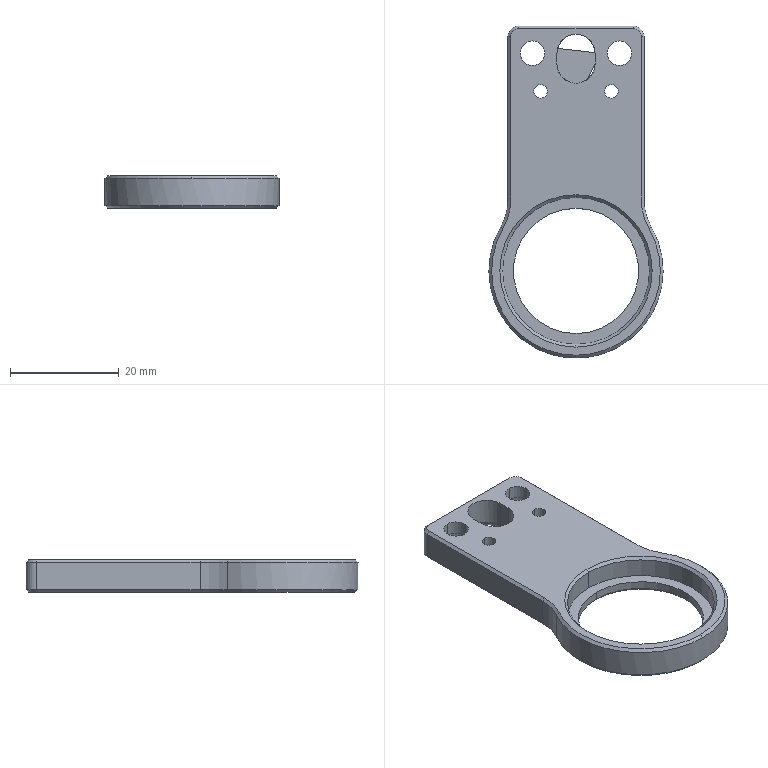NC program | NX | posted with a generic post | part box 32 x 61 x 6 mm
Lines 1 to 1417 of 12533:
N10 G17 G21 G94 G90
(FLOOR_WALL_COPY , TOOL : D80)
N12 T19 M6
N14 G54
N16 G17 G0 G90 X-106. Y0. S5000 M3
N18 G43 Z30. H19
N20 Z7.02
N22 G94 G1 Z4.02 F2000.
N24 X-101.
N26 X40.
N28 X45.
N30 Z7.02
N32 G0 Z30.
N34 X-106.
N36 Z6.04
N38 G1 Z3.04
N40 X-101.
N42 X40.
N44 X45.
N46 Z6.04
N48 G0 Z30.
N50 X-106.
N52 Z5.06
N54 G1 Z2.06
N56 X-101.
N58 X40.
N60 X45.
N62 Z5.06
N64 G0 Z30.
N66 X-106.
N68 Z4.08
N70 G1 Z1.08
N72 X-101.
N74 X40.
N76 X45.
N78 Z4.08
N80 G0 Z30.
N82 X-106.
N84 Z3.1
N86 G1 Z0.1
N88 X-101.
N90 X40.
N92 X45.
N94 Z3.1
N96 G0 Z30.
(FLOOR_WALL_COPY_COPY , TOOL : D80)
N98 X-106.
N100 Z3.
N102 G1 Z0. F1200.
N104 X-101.
N106 X40.
N108 X45.
N110 Z3.
N112 G0 Z30.
N114 M5
(HOLE_MILLING_2 , TOOL : D4)
N116 T11 M6
N118 G54
N120 G17 G0 G90 X-5. Y8. S9500 M3
N122 G43 Z30. H11
N124 Z0.5
N126 G94 G3 X-4.25 Y8.75 R0.75 F1250.
N128 X-5. Y9.5 R0.75
N130 X-5. Y9.5 Z0.1 I0. J-1.5
N132 X-5. Y9.5 Z-0.3 I0. J-1.5
N134 X-5. Y9.5 Z-0.7 I0. J-1.5
N136 X-5. Y9.5 Z-1.1 I0. J-1.5
N138 X-5. Y9.5 Z-1.5 I0. J-1.5
N140 X-5. Y9.5 Z-1.9 I0. J-1.5
N142 X-5. Y9.5 Z-2.3 I0. J-1.5
N144 X-5. Y9.5 Z-2.7 I0. J-1.5
N146 X-5. Y9.5 Z-3.1 I0. J-1.5
N148 X-5. Y9.5 Z-3.5 I0. J-1.5
N150 X-6.5 Y8. R1.5
N152 X-5. Y9.5 R-1.5
N154 X-5.75 Y8.75 R0.75
N156 X-5. Y8. R0.75
N158 G0 Z30.
N160 Y-8.
N162 Z0.5
N164 G3 X-4.25 Y-7.25 R0.75
N166 X-5. Y-6.5 R0.75
N168 X-5. Y-6.5 Z0.1 I0. J-1.5
N170 X-5. Y-6.5 Z-0.3 I0. J-1.5
N172 X-5. Y-6.5 Z-0.7 I0. J-1.5
N174 X-5. Y-6.5 Z-1.1 I0. J-1.5
N176 X-5. Y-6.5 Z-1.5 I0. J-1.5
N178 X-5. Y-6.5 Z-1.9 I0. J-1.5
N180 X-5. Y-6.5 Z-2.3 I0. J-1.5
N182 X-5. Y-6.5 Z-2.7 I0. J-1.5
N184 X-5. Y-6.5 Z-3.1 I0. J-1.5
N186 X-5. Y-6.5 Z-3.5 I0. J-1.5
N188 X-6.5 Y-8. R1.5
N190 X-5. Y-6.5 R-1.5
N192 X-5.75 Y-7.25 R0.75
N194 X-5. Y-8. R0.75
N196 G0 Z30.
(ZLEVEL_PROFILE_COPY_1 , TOOL : D4)
N198 X-20.254 Y1.745
N200 Z1.5
N202 G1 X-23.172 Z1.347 F1000.
N204 X-23.566 Y1.756 Z1.326
N206 X-24.329 Y1.54 Z1.285
N208 X-24.659 Y1.324 Z1.264
N210 Y-1.312 Z1.126
N212 X-24.347 Y-1.531 Z1.106
N214 X-23.552 Y-1.762 Z1.063
N216 X-23.172 Y-1.745 Z1.043
N218 X-4.675 Z0.073
N220 X-4.014 Y-1.476 Z0.036
N222 X-3.512 Y-0.968 Z-0.001
N224 X-3.251 Y-0.304 Z-0.039
N226 X-3.259 Y0.346 Z-0.073
N228 X-3.528 Y0.992 Z-0.11
N230 X-4.026 Y1.484 Z-0.146
N232 X-4.675 Y1.745 Z-0.183
N234 X-5. Z-0.2
N236 X-23.172 F2000.
N238 G3 X-24.659 Y1.324 R2.585
N240 G1 Y-1.312
N242 G3 X-23.172 Y-1.745 R2.404
N244 G1 X-5.
N246 G3 X-3.255 Y0. R1.745
N248 X-5. Y1.745 R1.745
N250 G1 X-6.817 Y1.737 Z-0.208
N252 X-8.634 Y1.729 Z-0.216
N254 X-10.451 Y1.721 Z-0.223
N256 X-12.269 Y1.713 Z-0.231
N258 X-14.086 Y1.706 Z-0.239
N260 X-15.903 Y1.699 Z-0.247
N262 X-17.72 Y1.691 Z-0.254
N264 X-19.537 Y1.684 Z-0.262
N266 X-21.354 Y1.677 Z-0.27
N268 X-23.172 Y1.674 Z-0.278
N270 X-23.696 Y1.617 Z-0.28
N272 X-23.928 Y1.577 Z-0.281
N274 X-24.446 Y1.356 Z-0.283
N276 X-24.575 Y1.296 Z-0.284
N278 X-24.564 Y-1.283 Z-0.295
N280 X-24.164 Y-1.474 Z-0.297
N282 X-23.916 Y-1.557 Z-0.298
N284 X-23.677 Y-1.612 Z-0.299
N286 X-23.172 Y-1.661 Z-0.301
N288 X-21.355 Y-1.644 Z-0.309
N290 X-19.537 Y-1.638 Z-0.317
N292 X-17.72 Y-1.632 Z-0.324
N294 X-15.903 Y-1.626 Z-0.332
N296 X-14.086 Y-1.62 Z-0.34
N298 X-12.269 Y-1.614 Z-0.348
N300 X-10.451 Y-1.609 Z-0.355
N302 X-8.634 Y-1.603 Z-0.363
N304 X-6.817 Y-1.598 Z-0.371
N306 X-5. Y-1.592 Z-0.379
N308 X-4.667 Y-1.556 Z-0.38
N310 X-4.505 Y-1.512 Z-0.381
N312 X-4.229 Y-1.39 Z-0.382
N314 X-4.06 Y-1.281 Z-0.383
N316 X-3.84 Y-1.085 Z-0.384
N318 X-3.709 Y-0.924 Z-0.385
N320 X-3.561 Y-0.67 Z-0.386
N322 X-3.487 Y-0.476 Z-0.387
N324 X-3.426 Y-0.189 Z-0.389
N326 X-3.415 Y0.019 Z-0.39
N328 X-3.446 Y0.306 Z-0.391
N330 X-3.499 Y0.504 Z-0.392
N332 X-3.616 Y0.767 Z-0.393
N334 X-3.727 Y0.939 Z-0.394
N336 X-3.919 Y1.154 Z-0.395
N338 X-4.077 Y1.283 Z-0.396
N340 X-4.325 Y1.429 Z-0.397
N342 X-4.516 Y1.503 Z-0.398
N344 X-4.755 Y1.56 Z-0.399
N346 X-5. Y1.578 Z-0.4
N348 X-6.817 Y1.573 Z-0.408
N350 X-8.634 Y1.568 Z-0.416
N352 X-10.451 Y1.563 Z-0.424
N354 X-12.269 Y1.558 Z-0.432
N356 X-14.086 Y1.553 Z-0.44
N358 X-15.903 Y1.549 Z-0.447
N360 X-17.72 Y1.544 Z-0.455
N362 X-19.537 Y1.54 Z-0.463
N364 X-21.355 Y1.535 Z-0.471
N366 X-23.174 Y1.533 Z-0.479
N368 X-23.59 Y1.504 Z-0.481
N370 X-23.823 Y1.45 Z-0.482
N372 X-24.321 Y1.279 Z-0.484
N374 X-24.374 Y1.251 Z-0.485
N376 X-24.363 Y-1.247 Z-0.495
N378 X-24.28 Y-1.299 Z-0.496
N380 X-23.822 Y-1.44 Z-0.498
N382 X-23.498 Y-1.491 Z-0.499
N384 X-23.172 Y-1.521 Z-0.501
N386 X-21.354 Y-1.516 Z-0.509
N388 X-19.537 Y-1.512 Z-0.517
N390 X-17.72 Y-1.508 Z-0.524
N392 X-15.903 Y-1.504 Z-0.532
N394 X-14.086 Y-1.501 Z-0.54
N396 X-12.269 Y-1.497 Z-0.548
N398 X-10.451 Y-1.494 Z-0.556
N400 X-8.634 Y-1.49 Z-0.564
N402 X-6.817 Y-1.487 Z-0.572
N404 X-5. Y-1.483 Z-0.58
N406 X-4.691 Y-1.45 Z-0.581
N408 X-4.541 Y-1.41 Z-0.582
N410 X-4.285 Y-1.298 Z-0.583
N412 X-4.127 Y-1.197 Z-0.584
N414 X-3.922 Y-1.016 Z-0.585
N416 X-3.8 Y-0.868 Z-0.586
N418 X-3.662 Y-0.633 Z-0.587
N420 X-3.591 Y-0.453 Z-0.588
N422 X-3.532 Y-0.187 Z-0.589
N424 X-3.521 Y0.006 Z-0.59
N426 X-3.547 Y0.275 Z-0.591
N428 X-3.595 Y0.461 Z-0.592
N430 X-3.703 Y0.709 Z-0.593
N432 X-3.807 Y0.871 Z-0.594
N434 X-3.986 Y1.074 Z-0.595
N436 X-4.134 Y1.196 Z-0.596
N438 X-4.367 Y1.334 Z-0.597
N440 X-4.545 Y1.404 Z-0.598
N442 X-4.77 Y1.458 Z-0.599
N444 X-5. Y1.475 Z-0.6
N446 X-6.817 Y1.472 Z-0.608
N448 X-8.634 Y1.469 Z-0.616
N450 X-10.451 Y1.466 Z-0.624
N452 X-12.269 Y1.463 Z-0.632
N454 X-14.086 Y1.461 Z-0.64
N456 X-15.903 Y1.458 Z-0.648
N458 X-17.72 Y1.455 Z-0.656
N460 X-19.537 Y1.453 Z-0.664
N462 X-21.354 Y1.45 Z-0.672
N464 X-23.172 Y1.448 Z-0.68
N466 X-23.219 Y1.454
N468 X-23.496 Y1.433 Z-0.682
N470 X-23.724 Y1.403 Z-0.683
N472 X-23.901 Y1.349
N474 X-24.076 Y1.289 Z-0.684
N476 X-24.174 Y1.243 Z-0.685
N478 X-24.168 Y-0.012 Z-0.69
N480 X-24.162 Y-1.244 Z-0.696
N482 X-24.071 Y-1.281
N484 X-23.898 Y-1.345 Z-0.697
N486 X-23.723 Y-1.398 Z-0.698
N488 X-23.449 Y-1.434 Z-0.699
N490 X-23.173 Y-1.443 Z-0.7
N492 X-21.355 Y-1.439 Z-0.708
N494 X-19.537 Y-1.437 Z-0.716
N496 X-17.72 Y-1.435 Z-0.724
N498 X-15.903 Y-1.433 Z-0.732
N500 X-14.086 Y-1.431 Z-0.74
N502 X-12.269 Y-1.429 Z-0.748
N504 X-10.451 Y-1.427 Z-0.756
N506 X-8.634 Y-1.426 Z-0.764
N508 X-6.817 Y-1.424 Z-0.772
N510 X-5. Y-1.422 Z-0.78
N512 X-4.634 Y-1.374 Z-0.782
N514 X-4.458 Y-1.314 Z-0.783
N516 X-4.168 Y-1.152 Z-0.784
N518 X-3.998 Y-1.008 Z-0.785
N520 X-3.796 Y-0.754 Z-0.787
N522 X-3.69 Y-0.55 Z-0.788
N524 X-3.6 Y-0.238 Z-0.789
N526 X-3.58 Y-0.009 Z-0.79
N528 X-3.616 Y0.316 Z-0.792
N530 X-3.686 Y0.537 Z-0.793
N532 X-3.843 Y0.823 Z-0.794
N534 X-3.993 Y1. Z-0.795
N536 X-4.248 Y1.204 Z-0.797
N538 X-4.455 Y1.31 Z-0.798
N540 X-4.722 Y1.391 Z-0.799
N542 X-5. Y1.418 Z-0.8
N544 X-6.827 Y1.417 Z-0.808
N546 X-8.653 Y1.415 Z-0.816
N548 X-10.48 Y1.414 Z-0.824
N550 X-12.307 Y1.413 Z-0.833
N552 X-14.133 Y1.412 Z-0.841
N554 X-15.96 Y1.41 Z-0.849
N556 X-17.787 Y1.409 Z-0.857
N558 X-19.613 Y1.408 Z-0.865
N560 X-21.356 Y1.407 Z-0.873
N562 X-23.098 Y1.406 Z-0.881
N564 X-23.182 Y1.414
N566 X-23.266 Y1.409
N568 X-23.466 Y1.383 Z-0.882
N570 X-23.665 Y1.35 Z-0.883
N572 X-23.931 Y1.263 Z-0.885
N574 X-23.974 Y1.245
N576 X-23.963 Y-1.245 Z-0.896
N578 X-23.909 Y-1.268
N580 X-23.617 Y-1.355 Z-0.897
N582 X-23.396 Y-1.391 Z-0.898
N584 X-23.064 Y-1.405 Z-0.9
N586 X-21.301 Y-1.404 Z-0.908
N588 X-19.537 Y-1.403 Z-0.916
N590 X-17.72 Z-0.924
N592 X-15.903 Y-1.402 Z-0.932
N594 X-14.086 Z-0.94
N596 X-12.269 Y-1.401 Z-0.948
N598 X-10.451 Z-0.956
N600 X-8.634 Z-0.964
N602 X-6.817 Y-1.4 Z-0.972
N604 X-5. Z-0.98
N606 X-4.638 Y-1.353 Z-0.982
N608 X-4.465 Y-1.294 Z-0.983
N610 X-4.178 Y-1.133 Z-0.984
N612 X-4.011 Y-0.991 Z-0.985
N614 X-3.81 Y-0.738 Z-0.987
N616 X-3.707 Y-0.537 Z-0.988
N618 X-3.619 Y-0.228 Z-0.989
N620 X-3.6 Y-0.002 Z-0.99
N622 X-3.636 Y0.317 Z-0.992
N624 X-3.706 Y0.535 Z-0.993
N626 X-3.862 Y0.815 Z-0.994
N628 X-4.009 Y0.989 Z-0.995
N630 X-4.261 Y1.189 Z-0.997
N632 X-4.464 Y1.293 Z-0.998
N634 X-5. Y1.401 Z-1.
N636 X-6.81 Y1.4 Z-1.008
N638 X-23.098 Z-1.081
N640 X-23.287 Y1.368 Z-1.082
N642 X-23.475 Y1.328 Z-1.083
N644 X-23.774 Y1.242 Z-1.085
N646 X-23.763 Y-1.234 Z-1.096
N648 X-23.732 Y-1.253
N650 X-23.459 Y-1.331 Z-1.097
N652 X-23.262 Y-1.369 Z-1.098
N654 X-23.064 Y-1.4 Z-1.099
N656 X-22.931 Z-1.1
N658 X-5. Z-1.18
N660 X-4.638 Y-1.352 Z-1.182
N662 X-4.464 Y-1.293 Z-1.183
N664 X-4.178 Y-1.133 Z-1.184
N666 X-4.01 Y-0.99 Z-1.185
N668 X-3.81 Y-0.738 Z-1.187
N670 X-3.707 Y-0.536 Z-1.188
N672 X-3.619 Y-0.227 Z-1.189
N674 X-3.6 Y0. Z-1.19
N676 X-3.637 Y0.319 Z-1.192
N678 X-3.707 Y0.536 Z-1.193
N680 X-3.862 Y0.816 Z-1.194
N682 X-4.01 Y0.99 Z-1.195
N684 X-4.261 Y1.189 Z-1.197
N686 X-4.464 Y1.293 Z-1.198
N688 X-4.727 Y1.373 Z-1.199
N690 X-5. Y1.4 Z-1.2
N692 X-19.372 Z-1.265
N694 X-21.168 Z-1.273
N696 X-22.964 Y1.391 Z-1.282
N698 X-23.137 Y1.376
N700 X-23.311 Y1.33 Z-1.283
N702 X-23.574 Y1.238 Z-1.284
N704 X-23.563 Y-1.234 Z-1.296
N706 X-23.469 Y-1.267
N708 X-23.386 Y-1.306 Z-1.297
N710 X-23.297 Y-1.328
N712 X-22.93 Y-1.389 Z-1.299
N714 X-21.138 Y-1.4 Z-1.307
N716 X-19.345 Z-1.315
N718 X-8.586 Z-1.364
N720 X-6.793 Z-1.372
N722 X-5. Z-1.38
N724 X-4.624 Y-1.349 Z-1.382
N726 X-4.444 Y-1.285 Z-1.383
N728 X-4.149 Y-1.112 Z-1.384
N730 X-3.979 Y-0.958 Z-1.385
N732 X-3.783 Y-0.692 Z-1.387
N734 X-3.682 Y-0.473 Z-1.388
N736 X-3.611 Y-0.172 Z-1.389
N738 X-3.601 Y0.053 Z-1.39
N740 X-3.648 Y0.362 Z-1.392
N742 X-3.722 Y0.573 Z-1.393
N744 X-3.882 Y0.842 Z-1.394
N746 X-4.029 Y1.009 Z-1.395
N748 X-4.277 Y1.199 Z-1.397
N750 X-4.477 Y1.298 Z-1.398
N752 X-4.733 Y1.374 Z-1.399
N754 X-5. Y1.4 Z-1.4
N756 X-19.215 Z-1.465
N758 X-20.991 Z-1.473
N760 X-22.766 Y1.382 Z-1.481
N762 X-23.113 Y1.329 Z-1.483
N764 X-23.193 Y1.304
N766 X-23.273 Y1.278 Z-1.484
N768 X-23.374 Y1.237
N770 X-23.363 Y-1.237 Z-1.496
N772 X-23.272 Y-1.277
N774 X-22.827 Y-1.371 Z-1.498
N776 X-21.047 Y-1.4 Z-1.506
N778 X-19.266 Z-1.515
N780 X-8.566 Z-1.564
N782 X-6.783 Z-1.572
N784 X-5. Z-1.58
N786 X-4.624 Y-1.349 Z-1.582
N788 X-4.444 Y-1.285 Z-1.583
N790 X-4.149 Y-1.112 Z-1.584
N792 X-3.979 Y-0.958 Z-1.585
N794 X-3.783 Y-0.692 Z-1.587
N796 X-3.682 Y-0.473 Z-1.588
N798 X-3.611 Y-0.172 Z-1.589
N800 X-3.601 Y0.053 Z-1.59
N802 X-3.648 Y0.362 Z-1.592
N804 X-3.722 Y0.573 Z-1.593
N806 X-3.882 Y0.842 Z-1.594
N808 X-4.029 Y1.009 Z-1.595
N810 X-4.277 Y1.199 Z-1.597
N812 X-4.477 Y1.298 Z-1.598
N814 X-4.733 Y1.374 Z-1.599
N816 X-5. Y1.4 Z-1.6
N818 X-18.938 Z-1.664
N820 X-20.68 Z-1.673
N822 X-22.421 Y1.387 Z-1.681
N824 X-22.842 Y1.339 Z-1.683
N826 X-22.96 Y1.319
N828 X-23.174 Y1.237 Z-1.684
N830 X-23.163 Y-1.236 Z-1.696
N832 X-23.069 Y-1.275
N834 X-22.951 Y-1.318 Z-1.697
N836 X-22.827 Y-1.338
N838 X-22.389 Y-1.39 Z-1.699
N840 X-20.651 Y-1.4 Z-1.707
N842 X-18.912 Z-1.715
N844 X-8.478 Z-1.764
N846 X-6.739 Z-1.772
N848 X-5. Z-1.78
N850 X-4.624 Y-1.349 Z-1.782
N852 X-4.444 Y-1.285
N854 X-4.149 Y-1.112 Z-1.784
N856 X-3.979 Y-0.958 Z-1.785
N858 X-3.783 Y-0.692 Z-1.787
N860 X-3.682 Y-0.473 Z-1.788
N862 X-3.611 Y-0.172 Z-1.789
N864 X-3.601 Y0.053 Z-1.79
N866 X-3.648 Y0.362 Z-1.792
N868 X-3.722 Y0.573 Z-1.793
N870 X-3.882 Y0.842 Z-1.794
N872 X-4.029 Y1.009 Z-1.795
N874 X-4.277 Y1.199 Z-1.797
N876 X-4.477 Y1.298 Z-1.798
N878 X-4.733 Y1.374 Z-1.799
N880 X-5. Y1.4 Z-1.8
N882 X-18.782 Z-1.864
N884 X-20.504 Z-1.872
N886 X-22.224 Y1.375 Z-1.88
N888 X-22.434 Y1.35 Z-1.881
N890 X-22.644 Y1.329 Z-1.882
N892 X-22.931 Y1.257 Z-1.884
N894 X-22.975 Y1.236
N896 X-22.969 Y-0.047 Z-1.89
N898 X-22.961 Y-1.24 Z-1.896
N900 X-22.917 Y-1.257
N902 X-22.53 Y-1.337 Z-1.898
N904 X-22.265 Y-1.367 Z-1.899
N906 X-21.999 Y-1.386 Z-1.9
N908 X-20.3 Y-1.4 Z-1.908
N910 X-18.6 Z-1.916
N912 X-8.4 Z-1.964
N914 X-6.7 Z-1.972
N916 X-5. Z-1.98
N918 X-4.624 Y-1.349 Z-1.981
N920 X-4.444 Y-1.285 Z-1.982
N922 X-4.149 Y-1.112 Z-1.984
N924 X-3.979 Y-0.958 Z-1.985
N926 X-3.783 Y-0.692 Z-1.986
N928 X-3.682 Y-0.473 Z-1.988
N930 X-3.611 Y-0.172 Z-1.989
N932 X-3.601 Y0.053 Z-1.99
N934 X-3.648 Y0.362 Z-1.991
N936 X-3.722 Y0.573 Z-1.993
N938 X-3.882 Y0.842 Z-1.994
N940 X-4.029 Y1.009 Z-1.995
N942 X-4.277 Y1.199 Z-1.996
N944 X-4.477 Y1.298 Z-1.998
N946 X-4.733 Y1.374 Z-1.999
N948 X-5. Y1.4 Z-2.
N950 X-6.288 Z-2.006
N952 X-7.576 Z-2.012
N954 X-7.961 Z-2.014
N956 X-8.346 Z-2.016
N958 X-10.019 Z-2.024
N960 X-11.692 Z-2.032
N962 X-13.365 Z-2.039
N964 X-15.037 Y1.399 Z-2.047
N966 X-16.71 Z-2.055
N968 X-18.383 Z-2.063
N970 X-19.675 Z-2.069
N972 X-20.967 Y1.392 Z-2.075
N974 X-21.347 Y1.384 Z-2.077
N976 X-21.728 Y1.369 Z-2.079
N978 X-22.015 Y1.356 Z-2.08
N980 X-22.297 Y1.338 Z-2.082
N982 X-22.714 Y1.252 Z-2.084
N984 X-22.775 Y1.227
N986 X-22.763 Y-1.225 Z-2.096
N988 X-22.703 Y-1.251
N990 X-22.296 Y-1.336 Z-2.098
N992 X-22.053 Y-1.351 Z-2.099
N994 X-21.727 Y-1.366 Z-2.1
N996 X-21.328 Y-1.381 Z-2.102
N998 X-20.929 Y-1.395 Z-2.104
N1000 X-19.656 Y-1.397 Z-2.11
N1002 X-18.383 Y-1.396 Z-2.116
N1004 X-16.71 Z-2.124
N1006 X-15.037 Y-1.395 Z-2.132
N1008 X-13.365 Z-2.14
N1010 X-11.692 Y-1.394 Z-2.148
N1012 X-10.019 Z-2.156
N1014 X-8.346 Y-1.393 Z-2.164
N1016 X-7.972 Z-2.165
N1018 X-7.598 Z-2.167
N1020 X-6.299 Y-1.4 Z-2.173
N1022 X-5. Z-2.179
N1024 X-4.624 Y-1.349 Z-2.181
N1026 X-4.444 Y-1.285 Z-2.182
N1028 X-4.149 Y-1.112 Z-2.184
N1030 X-3.979 Y-0.958 Z-2.185
N1032 X-3.783 Y-0.692 Z-2.186
N1034 X-3.682 Y-0.473 Z-2.187
N1036 X-3.611 Y-0.172 Z-2.189
N1038 X-3.601 Y0.053 Z-2.19
N1040 X-3.648 Y0.362 Z-2.191
N1042 X-3.722 Y0.573 Z-2.192
N1044 X-3.882 Y0.842 Z-2.194
N1046 X-4.029 Y1.009 Z-2.195
N1048 X-4.277 Y1.199 Z-2.196
N1050 X-4.477 Y1.298 Z-2.197
N1052 X-4.733 Y1.374 Z-2.199
N1054 X-5. Y1.4 Z-2.2
N1056 X-7.135 Z-2.21
N1058 X-7.355 Y1.389 Z-2.211
N1060 X-7.576 Y1.388 Z-2.212
N1062 X-7.761 Z-2.213
N1064 X-7.945 Z-2.214
N1066 X-9.427 Y1.387 Z-2.221
N1068 X-10.908 Y1.386 Z-2.228
N1070 X-12.574 Y1.385 Z-2.236
N1072 X-14.239 Y1.384 Z-2.244
N1074 X-15.905 Y1.383 Z-2.252
N1076 X-17.571 Y1.382 Z-2.26
N1078 X-19.236 Y1.381 Z-2.268
N1080 X-20.902 Y1.371 Z-2.276
N1082 X-21.405 Y1.354 Z-2.278
N1084 X-22.012 Y1.32 Z-2.281
N1086 X-22.505 Y1.231 Z-2.283
N1088 X-22.575 Y1.202 Z-2.284
N1090 X-22.563 Y-1.198 Z-2.295
N1092 X-22.499 Y-1.227 Z-2.296
N1094 X-22.049 Y-1.315 Z-2.298
N1096 X-21.954 Y-1.32
N1098 X-21.441 Y-1.35 Z-2.301
N1100 X-20.929 Y-1.361 Z-2.303
N1102 X-19.263 Y-1.374 Z-2.311
N1104 X-17.596 Y-1.373 Z-2.319
N1106 X-15.93 Y-1.372 Z-2.327
N1108 X-14.263 Y-1.37 Z-2.335
N1110 X-12.597 Y-1.369 Z-2.343
N1112 X-10.93 Y-1.367 Z-2.351
N1114 X-9.264 Y-1.366 Z-2.359
N1116 X-7.598 Y-1.372 Z-2.367
N1118 X-7.47 Y-1.378
N1120 X-7.343 Y-1.383 Z-2.368
N1122 X-7.225 Y-1.386 Z-2.369
N1124 X-7.108 Y-1.395
N1126 X-6.054 Y-1.4 Z-2.374
N1128 X-5. Z-2.379
N1130 X-4.624 Y-1.349 Z-2.381
N1132 X-4.444 Y-1.285 Z-2.382
N1134 X-4.149 Y-1.112 Z-2.383
N1136 X-3.979 Y-0.958 Z-2.385
N1138 X-3.783 Y-0.692 Z-2.386
N1140 X-3.682 Y-0.473 Z-2.387
N1142 X-3.611 Y-0.172 Z-2.389
N1144 X-3.601 Y0.053 Z-2.39
N1146 X-3.648 Y0.362 Z-2.391
N1148 X-3.722 Y0.573 Z-2.392
N1150 X-3.882 Y0.842 Z-2.394
N1152 X-4.029 Y1.009 Z-2.395
N1154 X-4.277 Y1.199 Z-2.396
N1156 X-4.477 Y1.298 Z-2.397
N1158 X-4.733 Y1.374 Z-2.399
N1160 X-5. Y1.4 Z-2.4
N1162 X-6.083 Z-2.405
N1164 X-7.165 Y1.389 Z-2.41
N1166 X-7.277 Y1.38 Z-2.411
N1168 X-7.572 Y1.37 Z-2.412
N1170 X-7.987 Y1.353 Z-2.414
N1172 X-8.236 Y1.354 Z-2.416
N1174 X-8.486 Z-2.417
N1176 X-9.851 Y1.352 Z-2.423
N1178 X-11.215 Y1.351 Z-2.43
N1180 X-12.83 Y1.349 Z-2.438
N1182 X-14.444 Y1.347 Z-2.446
N1184 X-16.058 Y1.345 Z-2.453
N1186 X-17.673 Y1.343 Z-2.461
N1188 X-19.287 Y1.341 Z-2.469
N1190 X-20.901 Y1.336 Z-2.477
N1192 X-21.403 Y1.313 Z-2.479
N1194 X-21.903 Y1.265 Z-2.482
N1196 X-22.335 Y1.184 Z-2.484
N1198 X-22.375 Y1.166
N1200 X-22.369 Y-0.034 Z-2.49
N1202 X-22.363 Y-1.162 Z-2.495
N1204 X-22.319 Y-1.182
N1206 X-21.945 Y-1.254 Z-2.497
N1208 X-21.438 Y-1.305 Z-2.5
N1210 X-20.929 Y-1.328 Z-2.502
N1212 X-19.231 Y-1.33 Z-2.51
N1214 X-17.532 Y-1.328 Z-2.518
N1216 X-15.834 Y-1.326 Z-2.527
N1218 X-14.136 Y-1.323 Z-2.535
N1220 X-12.438 Y-1.321 Z-2.543
N1222 X-10.739 Y-1.318 Z-2.551
N1224 X-9.612 Y-1.317 Z-2.557
N1226 X-8.484 Y-1.313 Z-2.562
N1228 X-7.914 Y-1.328 Z-2.565
N1230 X-7.345 Y-1.374 Z-2.568
N1232 X-7.172 Y-1.387
N1234 X-7. Y-1.4 Z-2.569
N1236 X-5. Z-2.579
N1238 X-4.624 Y-1.349 Z-2.581
N1240 X-4.444 Y-1.285 Z-2.582
N1242 X-4.149 Y-1.112 Z-2.583
N1244 X-3.979 Y-0.958 Z-2.584
N1246 X-3.783 Y-0.692 Z-2.586
N1248 X-3.682 Y-0.473 Z-2.587
N1250 X-3.611 Y-0.172 Z-2.589
N1252 X-3.601 Y0.053 Z-2.59
N1254 X-3.648 Y0.362 Z-2.591
N1256 X-3.722 Y0.573 Z-2.592
N1258 X-3.882 Y0.842 Z-2.594
N1260 X-4.029 Y1.009 Z-2.595
N1262 X-4.277 Y1.199 Z-2.596
N1264 X-4.477 Y1.298 Z-2.597
N1266 X-4.733 Y1.374 Z-2.599
N1268 X-5. Y1.4 Z-2.6
N1270 X-6.109 Z-2.605
N1272 X-7.217 Y1.38 Z-2.611
N1274 X-7.363 Y1.364 Z-2.612
N1276 X-7.613 Y1.334 Z-2.613
N1278 X-7.987 Y1.314 Z-2.615
N1280 X-8.236 Y1.306 Z-2.616
N1282 X-8.486 Y1.298 Z-2.617
N1284 X-8.735 Y1.297 Z-2.618
N1286 X-8.985 Y1.296 Z-2.62
N1288 X-10.291 Y1.294 Z-2.626
N1290 X-11.597 Y1.292 Z-2.632
N1292 X-13.152 Y1.289 Z-2.64
N1294 X-14.707 Y1.286 Z-2.647
N1296 X-16.263 Y1.284 Z-2.655
N1298 X-17.818 Y1.281 Z-2.663
N1300 X-19.373 Y1.278 Z-2.67
N1302 X-20.929 Y1.268 Z-2.678
N1304 X-21.26 Y1.257 Z-2.679
N1306 X-21.589 Y1.221 Z-2.681
N1308 X-22.126 Y1.128 Z-2.684
N1310 X-22.16 Y1.112
N1312 X-22.153 Y-0.042 Z-2.69
N1314 X-22.147 Y-1.109 Z-2.695
N1316 X-22.093 Y-1.13
N1318 X-21.589 Y-1.217 Z-2.698
N1320 X-21.26 Y-1.252 Z-2.699
N1322 X-20.929 Y-1.259 Z-2.701
N1324 X-19.373 Y-1.263 Z-2.708
N1326 X-17.818 Y-1.26 Z-2.716
N1328 X-16.262 Y-1.257 Z-2.724
N1330 X-14.707 Y-1.254 Z-2.731
N1332 X-13.151 Y-1.25 Z-2.739
N1334 X-11.595 Y-1.247 Z-2.746
N1336 X-10.29 Y-1.245 Z-2.753
N1338 X-8.985 Y-1.24 Z-2.759
N1340 X-8.482 Y-1.251 Z-2.762
N1342 X-7.829 Y-1.304 Z-2.765
N1344 X-7.179 Y-1.387 Z-2.768
N1346 X-7.09 Y-1.396
N1348 X-7. Y-1.4 Z-2.769
N1350 X-5. Z-2.779
N1352 X-4.624 Y-1.349 Z-2.78
N1354 X-4.444 Y-1.285 Z-2.781
N1356 X-4.149 Y-1.112 Z-2.783
N1358 X-3.979 Y-0.958 Z-2.784
N1360 X-3.783 Y-0.692 Z-2.786
N1362 X-3.682 Y-0.473 Z-2.787
N1364 X-3.611 Y-0.172 Z-2.788
N1366 X-3.601 Y0.053 Z-2.79
N1368 X-3.648 Y0.362 Z-2.791
N1370 X-3.722 Y0.573 Z-2.792
N1372 X-3.882 Y0.842 Z-2.794
N1374 X-4.029 Y1.009 Z-2.795
N1376 X-4.277 Y1.199 Z-2.796
N1378 X-4.477 Y1.298 Z-2.797
N1380 X-4.733 Y1.374 Z-2.799
N1382 X-5. Y1.4 Z-2.8
N1384 X-6.137 Z-2.806
N1386 X-7.271 Y1.373 Z-2.811
N1388 X-7.362 Y1.358 Z-2.812
N1390 X-7.472 Y1.351
N1392 X-7.654 Y1.307 Z-2.813
N1394 X-7.841 Y1.292 Z-2.814
N1396 X-7.985 Y1.275 Z-2.815
N1398 X-8.485 Y1.241 Z-2.817
N1400 X-8.985 Y1.211 Z-2.82
N1402 X-9.239 Y1.213 Z-2.821
N1404 X-9.493 Z-2.822
N1406 X-11.256 Y1.209 Z-2.831
N1408 X-13.02 Y1.204 Z-2.84
N1410 X-14.997 Y1.199 Z-2.85
N1412 X-16.974 Y1.194 Z-2.859
N1414 X-18.951 Y1.189 Z-2.869
N1416 X-20.928 Y1.171 Z-2.879
N1418 X-21.828 Y1.074 Z-2.883
N1420 X-21.916 Y1.045 Z-2.884
N1422 X-21.909 Y-0.01 Z-2.889
N1424 X-21.903 Y-1.041 Z-2.894
N1426 X-21.899 Y-1.05
N1428 X-21.719 Y-1.082 Z-2.895
N1430 X-21.472 Y-1.12 Z-2.897
N1432 X-21.201 Y-1.147 Z-2.898
N1434 X-20.929 Y-1.16 Z-2.899
N1436 X-18.938 Y-1.168 Z-2.909
N1438 X-16.948 Y-1.163 Z-2.919
N1440 X-14.957 Y-1.157 Z-2.929
N1442 X-12.966 Y-1.152 Z-2.939
N1444 X-11.23 Y-1.147 Z-2.947
N1446 X-9.494 Y-1.142 Z-2.956
N1448 X-8.981 Y-1.146 Z-2.958
N1450 X-8.543 Y-1.189 Z-2.961
N1452 X-8.105 Y-1.233 Z-2.963
N1454 X-7.769 Y-1.282 Z-2.965
N1456 X-7.434 Y-1.341 Z-2.966
N1458 X-7.337 Y-1.358 Z-2.967
N1460 X-7.241 Y-1.378
N1462 X-6.077 Y-1.4 Z-2.973
N1464 X-5. Z-2.978
N1466 X-4.624 Y-1.349 Z-2.98
N1468 X-4.444 Y-1.285 Z-2.981
N1470 X-4.149 Y-1.112 Z-2.983
N1472 X-3.979 Y-0.958 Z-2.984
N1474 X-3.783 Y-0.692 Z-2.986
N1476 X-3.682 Y-0.473 Z-2.987
N1478 X-3.611 Y-0.172 Z-2.988
N1480 X-3.601 Y0.053 Z-2.989
N1482 X-3.648 Y0.362 Z-2.991
N1484 X-3.722 Y0.573 Z-2.992
N1486 X-3.882 Y0.842 Z-2.994
N1488 X-4.029 Y1.009 Z-2.995
N1490 X-4.277 Y1.199 Z-2.996
N1492 X-4.477 Y1.298 Z-2.997
N1494 X-4.733 Y1.374 Z-2.999
N1496 X-5. Y1.4 Z-3.
N1498 X-6.175 Z-3.006
N1500 X-7.339 Y1.356 Z-3.012
N1502 X-7.474 Y1.34 Z-3.013
N1504 X-7.563 Y1.311
N1506 X-7.654 Y1.29 Z-3.014
N1508 X-8.064 Y1.228 Z-3.016
N1510 X-8.475 Y1.17 Z-3.018
N1512 X-8.983 Y1.126 Z-3.02
N1514 X-9.492 Y1.1 Z-3.023
N1516 X-9.752 Z-3.024
N1518 X-10.011 Z-3.025
N1520 X-11.658 Y1.094 Z-3.034
N1522 X-13.305 Y1.089 Z-3.042
N1524 X-15.211 Y1.082 Z-3.052
N1526 X-17.117 Y1.076 Z-3.061
N1528 X-19.023 Y1.069 Z-3.071
N1530 X-20.929 Y1.057 Z-3.081
N1532 X-21.568 Y0.984 Z-3.084
N1534 X-21.636 Y0.968
N1536 X-21.629 Y-0.005 Z-3.089
N1538 X-21.622 Y-0.963 Z-3.094
N1540 X-21.415 Y-0.99 Z-3.095
N1542 X-20.929 Y-1.046 Z-3.097
N1544 X-19.023 Y-1.044 Z-3.107
N1546 X-17.117 Y-1.037 Z-3.117
N1548 X-15.211 Y-1.03 Z-3.126
N1550 X-13.306 Y-1.023 Z-3.136
N1552 X-11.675 Y-1.017 Z-3.144
N1554 X-10.045 Y-1.011 Z-3.152
N1556 X-9.488 Y-1.015 Z-3.155
N1558 X-8.968 Y-1.064 Z-3.158
N1560 X-8.451 Y-1.128 Z-3.16
N1562 X-7.938 Y-1.216 Z-3.163
N1564 X-7.434 Y-1.34 Z-3.166
N1566 X-7.381 Y-1.345
N1568 X-7.332 Y-1.357
N1570 X-6.2 Y-1.4 Z-3.172
N1572 X-5. Z-3.178
N1574 X-4.624 Y-1.349 Z-3.18
N1576 X-4.444 Y-1.285 Z-3.181
N1578 X-4.149 Y-1.112 Z-3.183
N1580 X-3.979 Y-0.958 Z-3.184
N1582 X-3.783 Y-0.692 Z-3.185
N1584 X-3.682 Y-0.473 Z-3.187
N1586 X-3.611 Y-0.172 Z-3.188
N1588 X-3.601 Y0.053 Z-3.189
N1590 X-3.648 Y0.362 Z-3.191
N1592 X-3.722 Y0.573 Z-3.192
N1594 X-3.882 Y0.842 Z-3.193
N1596 X-4.029 Y1.009 Z-3.195
N1598 X-4.277 Y1.199 Z-3.196
N1600 X-4.477 Y1.298 Z-3.197
N1602 X-4.733 Y1.374 Z-3.199
N1604 X-5. Y1.4 Z-3.2
N1606 X-6.176 Z-3.206
N1608 X-7.345 Y1.355 Z-3.212
N1610 X-7.696 Y1.262 Z-3.214
N1612 X-8.271 Y1.155 Z-3.217
N1614 X-8.846 Y1.05 Z-3.22
N1616 X-9.561 Y0.957 Z-3.224
N1618 X-10.01 Y0.948 Z-3.226
N1620 X-10.266 Y0.95 Z-3.227
N1622 X-10.521 Y0.949 Z-3.229
N1624 X-12.086 Y0.942 Z-3.237
N1626 X-13.651 Y0.935 Z-3.245
N1628 X-15.47 Y0.927 Z-3.254
N1630 X-17.29 Y0.919 Z-3.264
N1632 X-19.109 Y0.91 Z-3.273
N1634 X-20.929 Y0.872 Z-3.282
N1636 X-21.307 Y0.864 Z-3.284
N1638 X-21.299 Y0.001 Z-3.289
N1640 X-21.289 Y-0.857 Z-3.293
N1642 X-20.929 Y-0.86 Z-3.295
N1644 X-19.115 Y-0.882 Z-3.304
N1646 X-17.301 Y-0.873 Z-3.314
N1648 X-15.487 Y-0.864 Z-3.323
N1650 X-13.673 Y-0.854 Z-3.332
N1652 X-12.099 Y-0.846 Z-3.341
N1654 X-10.525 Y-0.838 Z-3.349
N1656 X-10.036 Y-0.833 Z-3.351
N1658 X-9.37 Y-0.906 Z-3.355
N1660 X-8.71 Y-1.025 Z-3.358
N1662 X-8.155 Y-1.144 Z-3.361
N1664 X-7.603 Y-1.276 Z-3.364
N1666 X-7.474 Y-1.315 Z-3.365
N1668 X-7.345 Y-1.353
N1670 X-6.279 Y-1.4 Z-3.371
N1672 X-5. Z-3.377
N1674 X-4.624 Y-1.349 Z-3.379
N1676 X-4.444 Y-1.285 Z-3.38
N1678 X-4.149 Y-1.112 Z-3.382
N1680 X-3.979 Y-0.958 Z-3.383
N1682 X-3.783 Y-0.692 Z-3.385
N1684 X-3.682 Y-0.473 Z-3.386
N1686 X-3.611 Y-0.172 Z-3.388
N1688 X-3.601 Y0.053 Z-3.389
N1690 X-3.648 Y0.362 Z-3.391
N1692 X-3.722 Y0.573 Z-3.392
N1694 X-3.882 Y0.842 Z-3.393
N1696 X-4.029 Y1.009 Z-3.395
N1698 X-4.277 Y1.199 Z-3.396
N1700 X-4.477 Y1.298 Z-3.397
N1702 X-4.733 Y1.374 Z-3.399
N1704 X-5. Y1.4 Z-3.4
N1706 X-6.11 Z-3.406
N1708 X-7.219 Y1.38 Z-3.412
N1710 X-7.318 Y1.36
N1712 X-7.541 Y1.29 Z-3.414
N1714 X-8.006 Y1.159 Z-3.416
N1716 X-8.478 Y1.051 Z-3.419
N1718 X-9.552 Y0.825 Z-3.425
N1720 X-10.034 Y0.783 Z-3.427
N1722 X-10.516 Y0.745 Z-3.43
N1724 X-10.81 Y0.75 Z-3.431
N1726 X-11.104 Y0.748 Z-3.433
N1728 X-12.547 Y0.739 Z-3.441
N1730 X-13.99 Y0.73 Z-3.448
N1732 X-15.725 Y0.719 Z-3.457
N1734 X-17.46 Y0.708 Z-3.467
N1736 X-19.132 Y0.697 Z-3.475
N1738 X-20.805 Y0.686 Z-3.484
N1740 X-20.891 Y0.674 Z-3.485
N1742 X-20.903 Y0.665
N1744 X-20.894 Y-0.057 Z-3.489
N1746 X-20.887 Y-0.657 Z-3.492
N1748 X-20.876 Y-0.666
N1750 X-20.793 Y-0.676
N1752 X-19.127 Y-0.665 Z-3.501
N1754 X-17.461 Y-0.653 Z-3.51
N1756 X-15.727 Y-0.641 Z-3.519
N1758 X-13.993 Y-0.629 Z-3.528
N1760 X-12.549 Y-0.618 Z-3.536
N1762 X-11.106 Y-0.608 Z-3.544
N1764 X-10.506 Y-0.602 Z-3.547
N1766 X-9.784 Y-0.703 Z-3.551
N1768 X-9.071 Y-0.852 Z-3.555
N1770 X-8.405 Y-1.028 Z-3.558
N1772 X-7.742 Y-1.215 Z-3.562
N1774 X-7.67 Y-1.238
N1776 X-7.599 Y-1.264 Z-3.563
N1778 X-7.508 Y-1.3
N1780 X-7.417 Y-1.335 Z-3.564
N1782 X-7.243 Y-1.376 Z-3.565
N1784 X-7. Y-1.4 Z-3.566
N1786 X-5. Z-3.577
N1788 X-4.624 Y-1.349 Z-3.579
N1790 X-4.444 Y-1.285 Z-3.58
N1792 X-4.149 Y-1.112 Z-3.582
N1794 X-3.979 Y-0.958 Z-3.583
N1796 X-3.783 Y-0.692 Z-3.585
N1798 X-3.682 Y-0.473 Z-3.586
N1800 X-3.611 Y-0.172 Z-3.587
N1802 X-3.601 Y0.053 Z-3.589
N1804 X-3.648 Y0.362 Z-3.59
N1806 X-3.722 Y0.573 Z-3.592
N1808 X-3.882 Y0.842 Z-3.593
N1810 X-4.029 Y1.009 Z-3.594
N1812 X-4.277 Y1.199 Z-3.596
N1814 X-4.477 Y1.298 Z-3.597
N1816 X-4.733 Y1.374 Z-3.599
N1818 X-5. Y1.4 Z-3.6
N1820 X-6.11 Z-3.606
N1822 X-7.219 Y1.38 Z-3.612
N1824 X-7.351 Y1.353 Z-3.613
N1826 X-7.478 Y1.308 Z-3.614
N1828 X-8.085 Y1.102 Z-3.617
N1830 X-8.705 Y0.926 Z-3.621
N1832 X-9.289 Y0.762 Z-3.624
N1834 X-9.881 Y0.621 Z-3.628
N1836 X-10.331 Y0.533 Z-3.63
N1838 X-10.789 Y0.486 Z-3.633
N1840 X-11.093 Y0.463 Z-3.635
N1842 X-11.408 Y0.466 Z-3.636
N1844 X-11.724 Y0.463 Z-3.638
N1846 X-12.999 Y0.45 Z-3.645
N1848 X-14.275 Y0.438 Z-3.652
N1850 X-15.86 Y0.422 Z-3.661
N1852 X-17.446 Y0.406 Z-3.67
N1854 X-18.905 Y0.391 Z-3.678
N1856 X-20.362 Y0.373 Z-3.686
N1858 X-20.349 Y-0.366 Z-3.69
N1860 X-18.899 Y-0.353 Z-3.698
N1862 X-17.447 Y-0.337 Z-3.706
N1864 X-15.861 Y-0.319 Z-3.714
N1866 X-14.276 Y-0.3 Z-3.723
N1868 X-13.009 Y-0.285 Z-3.73
N1870 X-11.743 Y-0.269 Z-3.737
N1872 X-11.063 Y-0.286 Z-3.741
N1874 X-10.49 Y-0.369 Z-3.744
N1876 X-9.928 Y-0.502 Z-3.747
N1878 X-9.372 Y-0.655 Z-3.751
N1880 X-8.821 Y-0.821 Z-3.754
N1882 X-8.246 Y-1.028 Z-3.757
N1884 X-7.671 Y-1.235 Z-3.761
N1886 X-7.577 Y-1.273
N1888 X-7.482 Y-1.311 Z-3.762
N1890 X-7.254 Y-1.375 Z-3.763
N1892 X-7. Y-1.4 Z-3.765
N1894 X-5. Z-3.776
N1896 X-4.624 Y-1.349 Z-3.778
N1898 X-4.444 Y-1.285 Z-3.779
N1900 X-4.149 Y-1.112 Z-3.781
N1902 X-3.979 Y-0.958 Z-3.782
N1904 X-3.783 Y-0.692 Z-3.784
N1906 X-3.682 Y-0.473 Z-3.785
N1908 X-3.611 Y-0.172 Z-3.787
N1910 X-3.601 Y0.053 Z-3.788
N1912 X-3.648 Y0.362 Z-3.79
N1914 X-3.722 Y0.573 Z-3.791
N1916 X-3.882 Y0.842 Z-3.793
N1918 X-4.029 Y1.009 Z-3.794
N1920 X-4.277 Y1.199 Z-3.796
N1922 X-4.477 Y1.298 Z-3.797
N1924 X-4.733 Y1.374 Z-3.799
N1926 X-5. Y1.4 Z-3.8
N1928 X-6.11 Z-3.809
N1930 X-7.219 Y1.38 Z-3.818
N1932 X-7.285 Y1.368 Z-3.819
N1934 X-7.539 Y1.284 Z-3.821
N1936 X-8.33 Y0.976 Z-3.828
N1938 X-9.13 Y0.689 Z-3.835
N1940 X-9.505 Y0.554 Z-3.839
N1942 X-9.883 Y0.425 Z-3.842
N1944 X-10.546 Y0.214 Z-3.848
N1946 X-11.15 Y0.095 Z-3.855
N1948 X-10.941 Y0.042 Z-3.882
N1950 X-10.962 Y0.005 Z-3.889
N1952 X-10.834 Y-0.041 Z-3.892
N1954 X-10.347 Y-0.049 Z-3.906
N1956 X-10.241 Y-0.074 Z-3.916
N1958 X-10.021 Y-0.321 Z-3.921
N1960 X-9.445 Y-0.521 Z-3.925
N1962 X-8.888 Y-0.737 Z-3.93
N1964 X-8.21 Y-1.007 Z-3.936
N1966 X-7.537 Y-1.289 Z-3.942
N1968 X-7.268 Y-1.372 Z-3.945
N1970 X-7. Y-1.4 Z-3.947
N1972 X-5. Z-3.964
N1974 X-4.624 Y-1.349 Z-3.967
N1976 X-4.444 Y-1.285 Z-3.968
N1978 X-4.149 Y-1.112 Z-3.971
N1980 X-3.979 Y-0.958 Z-3.973
N1982 X-3.783 Y-0.692 Z-3.976
N1984 X-3.682 Y-0.473 Z-3.978
N1986 X-3.611 Y-0.172 Z-3.98
N1988 X-3.601 Y0.053 Z-3.982
N1990 X-3.648 Y0.362 Z-3.985
N1992 X-3.722 Y0.573 Z-3.987
N1994 X-3.882 Y0.842 Z-3.989
N1996 X-4.029 Y1.009 Z-3.991
N1998 X-4.277 Y1.199 Z-3.994
N2000 X-4.477 Y1.298 Z-3.996
N2002 X-4.733 Y1.374 Z-3.998
N2004 X-5. Y1.4 Z-4.
N2006 X-6.11 Z-4.015
N2008 X-7.219 Y1.38 Z-4.03
N2010 X-7.359 Y1.351 Z-4.032
N2012 X-7.601 Y1.26 Z-4.036
N2014 X-7.773 Y1.172 Z-4.038
N2016 X-7.947 Y1.088 Z-4.041
N2018 X-9.438 Y0.411 Z-4.063
N2020 X-9.657 Y0.303 Z-4.066
N2022 X-9.666 Y0.275 Z-4.067
N2024 X-9.67 Y0.196 Z-4.068
N2026 X-9.671 Y-0.011 Z-4.071
N2028 X-9.648 Y-0.272 Z-4.074
N2030 X-9.638 Y-0.303 Z-4.075
N2032 X-9.42 Y-0.408 Z-4.078
N2034 X-9.09 Y-0.557 Z-4.083
N2036 X-8.344 Y-0.907 Z-4.094
N2038 X-7.6 Y-1.263 Z-4.105
N2040 X-7.412 Y-1.338 Z-4.108
N2042 X-7.306 Y-1.364 Z-4.11
N2044 X-7.154 Y-1.39 Z-4.112
N2046 X-7. Y-1.4 Z-4.114
N2048 X-5. Z-4.141
N2050 X-4.624 Y-1.349 Z-4.146
N2052 X-4.444 Y-1.285 Z-4.149
N2054 X-4.149 Y-1.112 Z-4.153
N2056 X-3.979 Y-0.958 Z-4.156
N2058 X-3.783 Y-0.692 Z-4.161
N2060 X-3.682 Y-0.473 Z-4.164
N2062 X-3.611 Y-0.172 Z-4.168
N2064 X-3.601 Y0.053 Z-4.171
N2066 X-3.648 Y0.362 Z-4.175
N2068 X-3.722 Y0.573 Z-4.178
N2070 X-3.882 Y0.842 Z-4.183
N2072 X-4.029 Y1.009 Z-4.186
N2074 X-4.277 Y1.199 Z-4.19
N2076 X-4.477 Y1.298 Z-4.193
N2078 X-4.733 Y1.374 Z-4.196
N2080 X-5. Y1.4 Z-4.2
N2082 X-6.11 Z-4.216
N2084 X-7.219 Y1.38 Z-4.231
N2086 X-7.392 Y1.339 Z-4.234
N2088 X-7.665 Y1.23 Z-4.238
N2090 X-7.805 Y1.15 Z-4.24
N2092 X-7.869 Y1.132 Z-4.241
N2094 X-9.149 Y0.409 Z-4.262
N2096 X-9.295 Y0.325 Z-4.265
N2098 X-9.309 Y0.151 Z-4.267
N2100 X-9.311 Y0. Z-4.269
N2102 X-9.281 Y-0.323 Z-4.274
N2104 X-9.213 Y-0.364 Z-4.275
N2106 X-9.044 Y-0.469 Z-4.278
N2108 X-7.668 Y-1.229 Z-4.3
N2110 X-7.462 Y-1.318 Z-4.303
N2112 X-7.343 Y-1.355 Z-4.305
N2114 X-7.172 Y-1.386 Z-4.307
N2116 X-7. Y-1.4 Z-4.31
N2118 X-5. Z-4.338
N2120 X-4.624 Y-1.349 Z-4.343
N2122 X-4.444 Y-1.285 Z-4.346
N2124 X-4.149 Y-1.112 Z-4.351
N2126 X-3.979 Y-0.958 Z-4.354
N2128 X-3.783 Y-0.692 Z-4.359
N2130 X-3.682 Y-0.473 Z-4.362
N2132 X-3.611 Y-0.172 Z-4.367
N2134 X-3.601 Y0.053 Z-4.37
N2136 X-3.648 Y0.362 Z-4.374
N2138 X-3.722 Y0.573 Z-4.377
N2140 X-3.882 Y0.842 Z-4.382
N2142 X-4.029 Y1.009 Z-4.385
N2144 X-4.277 Y1.199 Z-4.389
N2146 X-4.477 Y1.298 Z-4.392
N2148 X-4.733 Y1.374 Z-4.396
N2150 X-5. Y1.4 Z-4.4
N2152 X-6.11 Z-4.416
N2154 X-7.219 Y1.38 Z-4.432
N2156 X-7.359 Y1.351 Z-4.435
N2158 X-7.748 Y1.181 Z-4.441
N2160 X-7.804 Y1.148 Z-4.442
N2162 X-7.864 Y1.121 Z-4.443
N2164 X-8.138 Y0.943 Z-4.447
N2166 X-8.415 Y0.77 Z-4.452
N2168 X-8.685 Y0.591 Z-4.457
N2170 X-8.951 Y0.405 Z-4.462
N2172 X-9.04 Y0.342 Z-4.463
N2174 X-9.059 Y0.165 Z-4.466
N2176 X-9.063 Y0. Z-4.468
N2178 X-9.04 Y-0.278 Z-4.472
N2180 X-9.032 Y-0.328 Z-4.473
N2182 X-9.021 Y-0.354
N2184 X-8.949 Y-0.409 Z-4.475
N2186 X-8.833 Y-0.485 Z-4.477
N2188 X-8.382 Y-0.776 Z-4.485
N2190 X-7.931 Y-1.066 Z-4.492
N2192 X-7.871 Y-1.104 Z-4.493
N2194 X-7.729 Y-1.193 Z-4.496
N2196 X-7.512 Y-1.299 Z-4.499
N2198 X-7.377 Y-1.346 Z-4.502
N2200 X-7.216 Y-1.381 Z-4.504
N2202 X-7. Y-1.4 Z-4.507
N2204 X-5. Z-4.536
N2206 X-4.624 Y-1.349 Z-4.542
N2208 X-4.444 Y-1.285 Z-4.545
N2210 X-4.149 Y-1.112 Z-4.549
N2212 X-3.979 Y-0.958 Z-4.553
N2214 X-3.783 Y-0.692 Z-4.558
N2216 X-3.682 Y-0.473 Z-4.561
N2218 X-3.611 Y-0.172 Z-4.566
N2220 X-3.601 Y0.053 Z-4.569
N2222 X-3.648 Y0.362 Z-4.573
N2224 X-3.722 Y0.573 Z-4.577
N2226 X-3.882 Y0.842 Z-4.581
N2228 X-4.029 Y1.009 Z-4.584
N2230 X-4.277 Y1.199 Z-4.589
N2232 X-4.477 Y1.298 Z-4.592
N2234 X-4.733 Y1.374 Z-4.596
N2236 X-5. Y1.4 Z-4.6
N2238 X-6.11 Z-4.617
N2240 X-7.219 Y1.38 Z-4.633
N2242 X-7.352 Y1.352 Z-4.635
N2244 X-7.525 Y1.29 Z-4.638
N2246 X-7.673 Y1.225 Z-4.64
N2248 X-7.811 Y1.141 Z-4.643
N2250 X-7.9 Y1.08 Z-4.644
N2252 X-7.988 Y1.018 Z-4.646
N2254 X-8.365 Y0.749 Z-4.653
N2256 X-8.578 Y0.597 Z-4.657
N2258 X-8.771 Y0.424 Z-4.661
N2260 X-8.848 Y0.352 Z-4.662
N2262 X-8.872 Y0.156 Z-4.665
N2264 X-8.877 Y-0.013 Z-4.668
N2266 X-8.851 Y-0.286 Z-4.672
N2268 X-8.84 Y-0.348 Z-4.673
N2270 X-8.825 Y-0.37
N2272 X-8.775 Y-0.421 Z-4.674
N2274 X-8.395 Y-0.721 Z-4.681
N2276 X-8. Y-1.007 Z-4.689
N2278 X-7.97 Y-1.043
N2280 X-7.927 Y-1.06 Z-4.69
N2282 X-7.868 Y-1.098 Z-4.691
N2284 X-7.812 Y-1.139 Z-4.692
N2286 X-7.567 Y-1.278 Z-4.696
N2288 X-7.424 Y-1.332 Z-4.699
N2290 X-7.238 Y-1.377 Z-4.701
N2292 X-7. Y-1.4 Z-4.705
N2294 X-5. Z-4.735
N2296 X-4.624 Y-1.349 Z-4.74
N2298 X-4.444 Y-1.285 Z-4.743
N2300 X-4.149 Y-1.112 Z-4.748
N2302 X-3.979 Y-0.958 Z-4.752
N2304 X-3.783 Y-0.692 Z-4.757
N2306 X-3.682 Y-0.473 Z-4.76
N2308 X-3.611 Y-0.172 Z-4.765
N2310 X-3.601 Y0.053 Z-4.768
N2312 X-3.648 Y0.362 Z-4.773
N2314 X-3.722 Y0.573 Z-4.776
N2316 X-3.882 Y0.842 Z-4.781
N2318 X-4.029 Y1.009 Z-4.784
N2320 X-4.277 Y1.199 Z-4.789
N2322 X-4.477 Y1.298 Z-4.792
N2324 X-4.733 Y1.374 Z-4.796
N2326 X-5. Y1.4 Z-4.8
N2328 X-6.11 Z-4.817
N2330 X-7.219 Y1.38 Z-4.834
N2332 X-7.369 Y1.347 Z-4.836
N2334 X-7.55 Y1.28 Z-4.839
N2336 X-7.709 Y1.206 Z-4.842
N2338 X-7.855 Y1.109 Z-4.844
N2340 X-7.918 Y1.059 Z-4.846
N2342 X-7.983 Y1.01 Z-4.847
N2344 X-8.629 Y0.455 Z-4.86
N2346 X-8.695 Y0.373 Z-4.861
N2348 X-8.714 Y0.266 Z-4.863
N2350 X-8.732 Y0. Z-4.867
N2352 X-8.702 Y-0.306 Z-4.872
N2354 X-8.679 Y-0.394 Z-4.873
N2356 X-8.619 Y-0.456 Z-4.874
N2358 X-7.994 Y-0.999 Z-4.887
N2360 X-7.925 Y-1.053 Z-4.888
N2362 X-7.857 Y-1.107 Z-4.89
N2364 X-7.609 Y-1.261 Z-4.894
N2366 X-7.451 Y-1.323 Z-4.897
N2368 X-7.249 Y-1.375 Z-4.9
N2370 X-7. Y-1.4 Z-4.903
N2372 X-5. Z-4.934
N2374 X-4.624 Y-1.349 Z-4.939
N2376 X-4.444 Y-1.285 Z-4.942
N2378 X-4.149 Y-1.112 Z-4.948
N2380 X-3.979 Y-0.958 Z-4.951
N2382 X-3.783 Y-0.692 Z-4.956
N2384 X-3.682 Y-0.473 Z-4.96
N2386 X-3.611 Y-0.172 Z-4.964
N2388 X-3.601 Y0.053 Z-4.968
N2390 X-3.648 Y0.362 Z-4.972
N2392 X-3.722 Y0.573 Z-4.976
N2394 X-3.882 Y0.842 Z-4.98
N2396 X-4.029 Y1.009 Z-4.984
N2398 X-4.277 Y1.199 Z-4.989
N2400 X-4.477 Y1.298 Z-4.992
N2402 X-4.733 Y1.374 Z-4.996
N2404 X-5. Y1.4 Z-5.
N2406 X-6.11 Z-5.017
N2408 X-7.219 Y1.379 Z-5.034
N2410 X-7.401 Y1.336 Z-5.037
N2412 X-7.589 Y1.264 Z-5.04
N2414 X-7.754 Y1.177 Z-5.043
N2416 X-7.921 Y1.054 Z-5.046
N2418 X-7.988 Y0.992 Z-5.048
N2420 X-8.146 Y0.868 Z-5.051
N2422 X-8.283 Y0.72 Z-5.054
N2424 X-8.435 Y0.559 Z-5.057
N2426 X-8.574 Y0.39 Z-5.061
N2428 X-8.598 Y0.274 Z-5.062
N2430 X-8.619 Y0. Z-5.067
N2432 X-8.591 Y-0.289 Z-5.071
N2434 X-8.57 Y-0.383 Z-5.073
N2436 X-8.446 Y-0.551 Z-5.076
N2438 X-8.377 Y-0.63 Z-5.077
N2440 X-8.232 Y-0.775 Z-5.081
N2442 X-7.923 Y-1.053 Z-5.087
N2444 X-7.661 Y-1.23 Z-5.092
N2446 X-7.49 Y-1.306 Z-5.095
N2448 X-7.275 Y-1.37 Z-5.098
N2450 X-7. Y-1.4 Z-5.102
N2452 X-5. Z-5.133
N2454 X-4.624 Y-1.349 Z-5.139
N2456 X-4.444 Y-1.285 Z-5.142
N2458 X-4.149 Y-1.112 Z-5.147
N2460 X-3.979 Y-0.958 Z-5.15
N2462 X-3.783 Y-0.692 Z-5.155
N2464 X-3.682 Y-0.473 Z-5.159
N2466 X-3.611 Y-0.172 Z-5.164
N2468 X-3.601 Y0.053 Z-5.167
N2470 X-3.648 Y0.362 Z-5.172
N2472 X-3.722 Y0.573 Z-5.175
N2474 X-3.882 Y0.842 Z-5.18
N2476 X-4.029 Y1.009 Z-5.184
N2478 X-4.277 Y1.199 Z-5.188
N2480 X-4.477 Y1.298 Z-5.192
N2482 X-4.733 Y1.374 Z-5.196
N2484 X-5. Y1.4 Z-5.2
N2486 X-6.11 Z-5.217
N2488 X-7.219 Y1.379 Z-5.234
N2490 X-7.434 Y1.323 Z-5.238
N2492 X-7.631 Y1.247 Z-5.241
N2494 X-7.782 Y1.159 Z-5.244
N2496 X-7.987 Y0.992 Z-5.248
N2498 X-8.059 Y0.92 Z-5.25
N2500 X-8.163 Y0.812 Z-5.252
N2502 X-8.268 Y0.705 Z-5.254
N2504 X-8.427 Y0.499 Z-5.258
N2506 X-8.468 Y0.429 Z-5.26
N2508 X-8.514 Y0.245 Z-5.262
N2510 X-8.532 Y-0.005 Z-5.266
N2512 X-8.504 Y-0.284 Z-5.271
N2514 X-8.473 Y-0.418 Z-5.273
N2516 X-8.287 Y-0.695 Z-5.278
N2518 X-8.169 Y-0.804 Z-5.28
N2520 X-7.99 Y-0.99 Z-5.284
N2522 X-7.714 Y-1.2 Z-5.29
N2524 X-7.533 Y-1.291 Z-5.293
N2526 X-7.306 Y-1.363 Z-5.297
N2528 X-7. Y-1.4 Z-5.301
N2530 X-5. Z-5.332
N2532 X-4.624 Y-1.349 Z-5.338
N2534 X-4.444 Y-1.285 Z-5.341
N2536 X-4.149 Y-1.112 Z-5.346
N2538 X-3.979 Y-0.958 Z-5.35
N2540 X-3.783 Y-0.692 Z-5.355
N2542 X-3.682 Y-0.473 Z-5.359
N2544 X-3.611 Y-0.172 Z-5.363
N2546 X-3.601 Y0.053 Z-5.367
N2548 X-3.648 Y0.362 Z-5.372
N2550 X-3.722 Y0.573 Z-5.375
N2552 X-3.882 Y0.842 Z-5.38
N2554 X-4.029 Y1.009 Z-5.383
N2556 X-4.277 Y1.199 Z-5.388
N2558 X-4.477 Y1.298 Z-5.392
N2560 X-4.733 Y1.374 Z-5.396
N2562 X-5. Y1.4 Z-5.4
N2564 X-6.11 Z-5.417
N2566 X-7.219 Y1.379 Z-5.435
N2568 X-7.464 Y1.312 Z-5.439
N2570 X-7.676 Y1.223 Z-5.442
N2572 X-7.843 Y1.117 Z-5.445
N2574 X-8.057 Y0.918 Z-5.45
N2576 X-8.134 Y0.828 Z-5.452
N2578 X-8.2 Y0.753 Z-5.453
N2580 X-8.263 Y0.676 Z-5.455
N2582 X-8.369 Y0.495 Z-5.458
N2584 X-8.415 Y0.401 Z-5.46
N2586 X-8.454 Y0.216 Z-5.463
N2588 X-8.469 Y-0.002 Z-5.466
N2590 X-8.446 Y-0.251 Z-5.47
N2592 X-8.412 Y-0.4 Z-5.472
N2594 X-8.264 Y-0.677 Z-5.477
N2596 X-8.199 Y-0.752 Z-5.479
N2598 X-8.059 Y-0.916 Z-5.482
N2600 X-7.882 Y-1.087 Z-5.486
N2602 X-7.755 Y-1.176 Z-5.488
N2604 X-7.542 Y-1.288 Z-5.492
N2606 X-7.393 Y-1.34 Z-5.495
N2608 X-7.221 Y-1.38 Z-5.497
N2610 X-7. Y-1.4 Z-5.501
N2612 X-5. Z-5.532
N2614 X-4.624 Y-1.349 Z-5.538
N2616 X-4.444 Y-1.285 Z-5.541
N2618 X-4.149 Y-1.112 Z-5.546
N2620 X-3.979 Y-0.958 Z-5.55
N2622 X-3.783 Y-0.692 Z-5.555
N2624 X-3.682 Y-0.473 Z-5.558
N2626 X-3.611 Y-0.172 Z-5.563
N2628 X-3.601 Y0.053 Z-5.567
N2630 X-3.648 Y0.362 Z-5.572
N2632 X-3.722 Y0.573 Z-5.575
N2634 X-3.882 Y0.842 Z-5.58
N2636 X-4.029 Y1.009 Z-5.583
N2638 X-4.277 Y1.199 Z-5.588
N2640 X-4.477 Y1.298 Z-5.592
N2642 X-4.733 Y1.374 Z-5.596
N2644 X-5. Y1.4 Z-5.6
N2646 X-6.11 Z-5.617
N2648 X-7.219 Y1.379 Z-5.635
N2650 X-7.499 Y1.3 Z-5.639
N2652 X-7.727 Y1.193 Z-5.643
N2654 X-7.907 Y1.064 Z-5.647
N2656 X-8.131 Y0.825 Z-5.652
N2658 X-8.174 Y0.762 Z-5.653
N2660 X-8.221 Y0.702 Z-5.654
N2662 X-8.387 Y0.427 Z-5.659
N2664 X-8.427 Y-0.002 Z-5.666
N2666 X-8.393 Y-0.304 Z-5.671
N2668 X-8.375 Y-0.452 Z-5.673
N2670 X-8.221 Y-0.701 Z-5.677
N2672 X-8.175 Y-0.76 Z-5.679
N2674 X-8.133 Y-0.822 Z-5.68
N2676 X-7.955 Y-1.024 Z-5.684
N2678 X-7.82 Y-1.131 Z-5.687
N2680 X-7.593 Y-1.264 Z-5.691
N2682 X-7.431 Y-1.329 Z-5.694
N2684 X-7.246 Y-1.377 Z-5.697
N2686 X-7. Y-1.4 Z-5.7
N2688 X-5. Z-5.732
N2690 X-4.624 Y-1.349 Z-5.738
N2692 X-4.444 Y-1.285 Z-5.741
N2694 X-4.149 Y-1.112 Z-5.746
N2696 X-3.979 Y-0.958 Z-5.749
N2698 X-3.783 Y-0.692 Z-5.755
N2700 X-3.682 Y-0.473 Z-5.758
N2702 X-3.611 Y-0.172 Z-5.763
N2704 X-3.601 Y0.053 Z-5.767
N2706 X-3.648 Y0.362 Z-5.772
N2708 X-3.722 Y0.573 Z-5.775
N2710 X-3.882 Y0.842 Z-5.78
N2712 X-4.029 Y1.009 Z-5.783
N2714 X-4.277 Y1.199 Z-5.788
N2716 X-4.477 Y1.298 Z-5.792
N2718 X-4.733 Y1.374 Z-5.796
N2720 X-5. Y1.4 Z-5.8
N2722 X-6.11 Z-5.817
N2724 X-7.22 Y1.379 Z-5.835
N2726 X-7.418 Y1.328 Z-5.838
N2728 X-7.611 Y1.254 Z-5.841
N2730 X-7.812 Y1.14 Z-5.845
N2732 X-7.952 Y1.021 Z-5.848
N2734 X-8.106 Y0.859 Z-5.851
N2736 X-8.213 Y0.697 Z-5.854
N2738 X-8.354 Y0.414 Z-5.859
N2740 X-8.384 Y0.242 Z-5.862
N2742 X-8.404 Y0. Z-5.866
N2744 X-8.381 Y-0.252 Z-5.87
N2746 X-8.354 Y-0.409 Z-5.872
N2748 X-8.296 Y-0.541 Z-5.875
N2750 X-8.212 Y-0.696 Z-5.877
N2752 X-8.025 Y-0.953 Z-5.882
N2754 X-7.902 Y-1.071 Z-5.885
N2756 X-7.67 Y-1.224 Z-5.889
N2758 X-7.478 Y-1.31 Z-5.893
N2760 X-7.271 Y-1.37 Z-5.896
N2762 X-7. Y-1.4 Z-5.9
N2764 X-5. Z-5.932
N2766 X-4.624 Y-1.349 Z-5.937
N2768 X-4.444 Y-1.285 Z-5.94
N2770 X-4.149 Y-1.112 Z-5.946
N2772 X-3.979 Y-0.958 Z-5.949
N2774 X-3.783 Y-0.692 Z-5.954
N2776 X-3.682 Y-0.473 Z-5.958
N2778 X-3.611 Y-0.172 Z-5.963
N2780 X-3.601 Y0.053 Z-5.967
N2782 X-3.648 Y0.362 Z-5.971
N2784 X-3.722 Y0.573 Z-5.975
N2786 X-3.882 Y0.842 Z-5.98
N2788 X-4.029 Y1.009 Z-5.983
N2790 X-4.277 Y1.199 Z-5.988
N2792 X-4.477 Y1.298 Z-5.992
N2794 X-4.733 Y1.374 Z-5.996
N2796 X-5. Y1.4 Z-6.
N2798 X-7.221
N2800 G3 X-8.343 Y0.396 R1.387
N2802 X-7. Y-1.4 R1.4
N2804 G1 X-5.
N2806 G3 X-3.6 Y0. R1.4
N2808 X-5. Y1.4 R1.4
N2810 G1 Z-4.5
N2812 G0 Z30.
N2814 M5